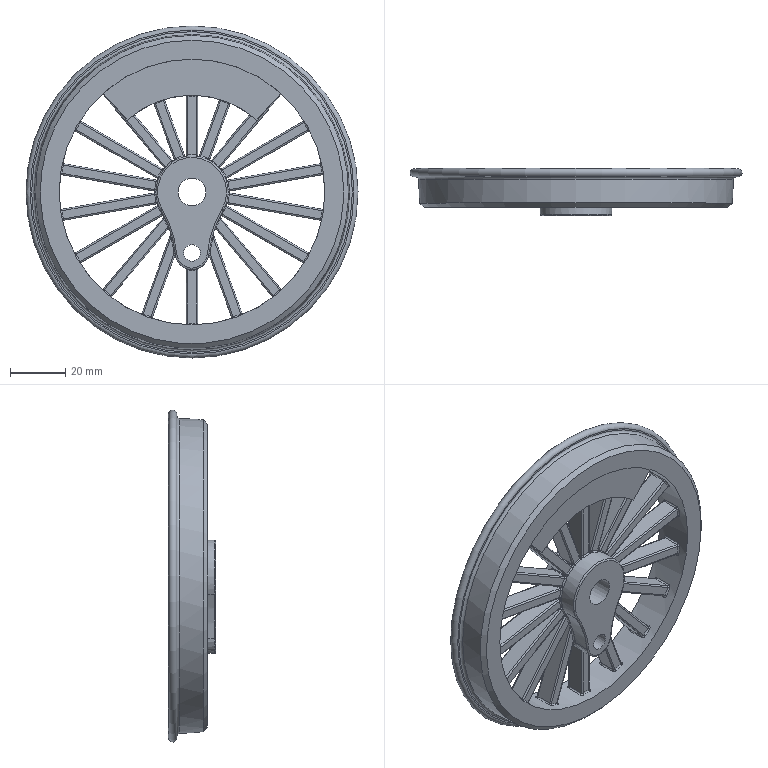Part | STEP file | 2-01.1 | 1 solid | 456 faces | box 120 x 17 x 120 mm | volume 77367 mm3 | spline 176 | cylinder 148 | plane 82 | torus 48 | cone 2 | commonest cylinder face diameters 1 x142 80 x2 6 x1 10 x1 70 x1 96 x1